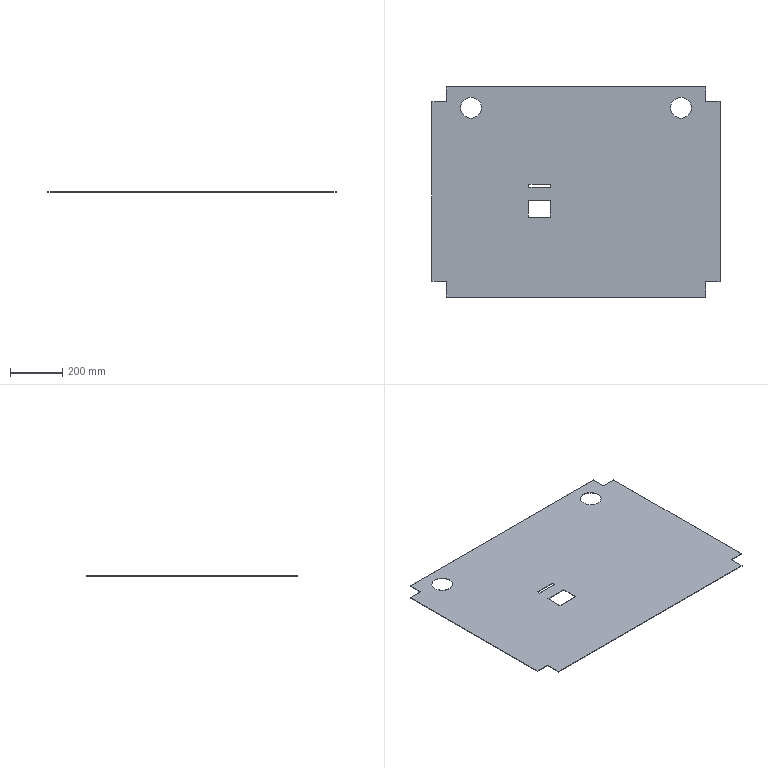Part | SolidWorks | features Cut 2, Extrusion 1 | 1 solid | 26 faces | box 1105 x 806 x 2 mm | volume 1722946 mm3 | plane 22 | cylinder 4 | commonest cylinder face diameters 80 x4
STEP:
#1=CARTESIAN_POINT('',(547.229,80.234,2.));
#2=VERTEX_POINT('',#1);
#3=CARTESIAN_POINT('',(627.229,80.234,2.));
#4=VERTEX_POINT('',#3);
#5=CARTESIAN_POINT('',(587.229,80.234,2.));
#6=DIRECTION('',(0.,0.,1.));
#7=DIRECTION('',(1.,0.,0.));
#8=AXIS2_PLACEMENT_3D('',#5,#6,#7);
#9=CIRCLE('',#8,40.);
#10=EDGE_CURVE('',#2,#4,#9,.T.);
#11=ORIENTED_EDGE('',*,*,#10,.T.);
#12=CARTESIAN_POINT('',(627.229,80.234,0.));
#13=VERTEX_POINT('',#12);
#14=CARTESIAN_POINT('',(627.229,80.234,2.));
#15=DIRECTION('',(0.,0.,-1.));
#16=VECTOR('',#15,1000.);
#17=LINE('',#14,#16);
#18=EDGE_CURVE('',#4,#13,#17,.T.);
#19=ORIENTED_EDGE('',*,*,#18,.T.);
#20=CARTESIAN_POINT('',(547.229,80.234,0.));
#21=VERTEX_POINT('',#20);
#22=CARTESIAN_POINT('',(587.229,80.234,0.));
#23=DIRECTION('',(0.,0.,1.));
#24=DIRECTION('',(1.,0.,0.));
#25=AXIS2_PLACEMENT_3D('',#22,#23,#24);
#26=CIRCLE('',#25,40.);
#27=EDGE_CURVE('',#21,#13,#26,.T.);
#28=ORIENTED_EDGE('',*,*,#27,.F.);
#29=CARTESIAN_POINT('',(547.229,80.234,2.));
#30=DIRECTION('',(0.,0.,-1.));
#31=VECTOR('',#30,1000.);
#32=LINE('',#29,#31);
#33=EDGE_CURVE('',#2,#21,#32,.T.);
#34=ORIENTED_EDGE('',*,*,#33,.F.);
#35=EDGE_LOOP('',(#11,#19,#28,#34));
#36=FACE_OUTER_BOUND('',#35,.T.);
#37=CARTESIAN_POINT('',(587.229,80.234,2.));
#38=DIRECTION('',(0.,0.,-1.));
#39=DIRECTION('',(-1.,0.,0.));
#40=AXIS2_PLACEMENT_3D('',#37,#38,#39);
#41=CYLINDRICAL_SURFACE('',#40,40.);
#42=ADVANCED_FACE('',(#36),#41,.F.);
#43=CARTESIAN_POINT('',(-257.771,80.234,2.));
#44=VERTEX_POINT('',#43);
#45=CARTESIAN_POINT('',(-177.771,80.234,2.));
#46=VERTEX_POINT('',#45);
#47=CARTESIAN_POINT('',(-217.771,80.234,2.));
#48=DIRECTION('',(0.,0.,1.));
#49=DIRECTION('',(1.,0.,0.));
#50=AXIS2_PLACEMENT_3D('',#47,#48,#49);
#51=CIRCLE('',#50,40.);
#52=EDGE_CURVE('',#44,#46,#51,.T.);
#53=ORIENTED_EDGE('',*,*,#52,.T.);
#54=CARTESIAN_POINT('',(-177.771,80.234,0.));
#55=VERTEX_POINT('',#54);
#56=CARTESIAN_POINT('',(-177.771,80.234,2.));
#57=DIRECTION('',(0.,0.,-1.));
#58=VECTOR('',#57,1000.);
#59=LINE('',#56,#58);
#60=EDGE_CURVE('',#46,#55,#59,.T.);
#61=ORIENTED_EDGE('',*,*,#60,.T.);
#62=CARTESIAN_POINT('',(-257.771,80.234,0.));
#63=VERTEX_POINT('',#62);
#64=CARTESIAN_POINT('',(-217.771,80.234,0.));
#65=DIRECTION('',(0.,0.,1.));
#66=DIRECTION('',(1.,0.,0.));
#67=AXIS2_PLACEMENT_3D('',#64,#65,#66);
#68=CIRCLE('',#67,40.);
#69=EDGE_CURVE('',#63,#55,#68,.T.);
#70=ORIENTED_EDGE('',*,*,#69,.F.);
#71=CARTESIAN_POINT('',(-257.771,80.234,2.));
#72=DIRECTION('',(0.,0.,-1.));
#73=VECTOR('',#72,1000.);
#74=LINE('',#71,#73);
#75=EDGE_CURVE('',#44,#63,#74,.T.);
#76=ORIENTED_EDGE('',*,*,#75,.F.);
#77=EDGE_LOOP('',(#53,#61,#70,#76));
#78=FACE_OUTER_BOUND('',#77,.T.);
#79=CARTESIAN_POINT('',(-217.771,80.234,2.));
#80=DIRECTION('',(0.,0.,-1.));
#81=DIRECTION('',(-1.,0.,0.));
#82=AXIS2_PLACEMENT_3D('',#79,#80,#81);
#83=CYLINDRICAL_SURFACE('',#82,40.);
#84=ADVANCED_FACE('',(#78),#83,.F.);
#85=CARTESIAN_POINT('',(1.292,-274.291,2.));
#86=VERTEX_POINT('',#85);
#87=CARTESIAN_POINT('',(86.292,-274.291,2.));
#88=VERTEX_POINT('',#87);
#89=CARTESIAN_POINT('',(46.292,-274.291,2.));
#90=DIRECTION('',(1.,0.,0.));
#91=VECTOR('',#90,1000.);
#92=LINE('',#89,#91);
#93=EDGE_CURVE('',#86,#88,#92,.T.);
#94=ORIENTED_EDGE('',*,*,#93,.T.);
#95=CARTESIAN_POINT('',(86.292,-339.291,2.));
#96=VERTEX_POINT('',#95);
#97=CARTESIAN_POINT('',(86.292,-274.291,2.));
#98=DIRECTION('',(0.,-1.,0.));
#99=VECTOR('',#98,1000.);
#100=LINE('',#97,#99);
#101=EDGE_CURVE('',#88,#96,#100,.T.);
#102=ORIENTED_EDGE('',*,*,#101,.T.);
#103=CARTESIAN_POINT('',(1.292,-339.291,2.));
#104=VERTEX_POINT('',#103);
#105=CARTESIAN_POINT('',(1.292,-339.291,2.));
#106=DIRECTION('',(-1.,0.,0.));
#107=VECTOR('',#106,1000.);
#108=LINE('',#105,#107);
#109=EDGE_CURVE('',#96,#104,#108,.T.);
#110=ORIENTED_EDGE('',*,*,#109,.T.);
#111=CARTESIAN_POINT('',(1.292,-274.291,2.));
#112=DIRECTION('',(0.,1.,0.));
#113=VECTOR('',#112,1000.);
#114=LINE('',#111,#113);
#115=EDGE_CURVE('',#104,#86,#114,.T.);
#116=ORIENTED_EDGE('',*,*,#115,.T.);
#117=EDGE_LOOP('',(#94,#102,#110,#116));
#118=FACE_BOUND('',#117,.T.);
#119=CARTESIAN_POINT('',(4.292,-225.291,2.));
#120=VERTEX_POINT('',#119);
#121=CARTESIAN_POINT('',(4.292,-213.291,2.));
#122=VERTEX_POINT('',#121);
#123=CARTESIAN_POINT('',(4.292,-225.291,2.));
#124=DIRECTION('',(0.,1.,0.));
#125=VECTOR('',#124,1000.);
#126=LINE('',#123,#125);
#127=EDGE_CURVE('',#120,#122,#126,.T.);
#128=ORIENTED_EDGE('',*,*,#127,.T.);
#129=CARTESIAN_POINT('',(86.292,-213.291,2.));
#130=VERTEX_POINT('',#129);
#131=CARTESIAN_POINT('',(4.292,-213.291,2.));
#132=DIRECTION('',(1.,0.,0.));
#133=VECTOR('',#132,1000.);
#134=LINE('',#131,#133);
#135=EDGE_CURVE('',#122,#130,#134,.T.);
#136=ORIENTED_EDGE('',*,*,#135,.T.);
#137=CARTESIAN_POINT('',(86.292,-225.291,2.));
#138=VERTEX_POINT('',#137);
#139=CARTESIAN_POINT('',(86.292,-213.291,2.));
#140=DIRECTION('',(0.,-1.,0.));
#141=VECTOR('',#140,1000.);
#142=LINE('',#139,#141);
#143=EDGE_CURVE('',#130,#138,#142,.T.);
#144=ORIENTED_EDGE('',*,*,#143,.T.);
#145=CARTESIAN_POINT('',(86.292,-225.291,2.));
#146=DIRECTION('',(-1.,0.,0.));
#147=VECTOR('',#146,1000.);
#148=LINE('',#145,#147);
#149=EDGE_CURVE('',#138,#120,#148,.T.);
#150=ORIENTED_EDGE('',*,*,#149,.T.);
#151=EDGE_LOOP('',(#128,#136,#144,#150));
#152=FACE_BOUND('',#151,.T.);
#153=ORIENTED_EDGE('',*,*,#52,.F.);
#154=CARTESIAN_POINT('',(-217.771,80.234,2.));
#155=DIRECTION('',(0.,0.,1.));
#156=DIRECTION('',(1.,0.,0.));
#157=AXIS2_PLACEMENT_3D('',#154,#155,#156);
#158=CIRCLE('',#157,40.);
#159=EDGE_CURVE('',#46,#44,#158,.T.);
#160=ORIENTED_EDGE('',*,*,#159,.F.);
#161=EDGE_LOOP('',(#153,#160));
#162=FACE_BOUND('',#161,.T.);
#163=CARTESIAN_POINT('',(-367.771,104.234,2.));
#164=VERTEX_POINT('',#163);
#165=CARTESIAN_POINT('',(-367.771,-585.766,2.));
#166=VERTEX_POINT('',#165);
#167=CARTESIAN_POINT('',(-367.771,104.234,2.));
#168=DIRECTION('',(0.,-1.,0.));
#169=VECTOR('',#168,1000.);
#170=LINE('',#167,#169);
#171=EDGE_CURVE('',#164,#166,#170,.T.);
#172=ORIENTED_EDGE('',*,*,#171,.T.);
#173=CARTESIAN_POINT('',(-312.771,-585.766,2.));
#174=VERTEX_POINT('',#173);
#175=CARTESIAN_POINT('',(-367.771,-585.766,2.));
#176=DIRECTION('',(1.,0.,0.));
#177=VECTOR('',#176,1000.);
#178=LINE('',#175,#177);
#179=EDGE_CURVE('',#166,#174,#178,.T.);
#180=ORIENTED_EDGE('',*,*,#179,.T.);
#181=CARTESIAN_POINT('',(-312.771,-645.766,2.));
#182=VERTEX_POINT('',#181);
#183=CARTESIAN_POINT('',(-312.771,-585.766,2.));
#184=DIRECTION('',(0.,-1.,0.));
#185=VECTOR('',#184,1000.);
#186=LINE('',#183,#185);
#187=EDGE_CURVE('',#174,#182,#186,.T.);
#188=ORIENTED_EDGE('',*,*,#187,.T.);
#189=CARTESIAN_POINT('',(682.229,-645.766,2.));
#190=VERTEX_POINT('',#189);
#191=CARTESIAN_POINT('',(-312.771,-645.766,2.));
#192=DIRECTION('',(1.,0.,0.));
#193=VECTOR('',#192,1000.);
#194=LINE('',#191,#193);
#195=EDGE_CURVE('',#182,#190,#194,.T.);
#196=ORIENTED_EDGE('',*,*,#195,.T.);
#197=CARTESIAN_POINT('',(682.229,-587.766,2.));
#198=VERTEX_POINT('',#197);
#199=CARTESIAN_POINT('',(682.229,-587.766,2.));
#200=DIRECTION('',(0.,1.,0.));
#201=VECTOR('',#200,1000.);
#202=LINE('',#199,#201);
#203=EDGE_CURVE('',#190,#198,#202,.T.);
#204=ORIENTED_EDGE('',*,*,#203,.T.);
#205=CARTESIAN_POINT('',(737.229,-587.766,2.));
#206=VERTEX_POINT('',#205);
#207=CARTESIAN_POINT('',(737.229,-587.766,2.));
#208=DIRECTION('',(1.,0.,0.));
#209=VECTOR('',#208,1000.);
#210=LINE('',#207,#209);
#211=EDGE_CURVE('',#198,#206,#210,.T.);
#212=ORIENTED_EDGE('',*,*,#211,.T.);
#213=CARTESIAN_POINT('',(737.229,105.234,2.));
#214=VERTEX_POINT('',#213);
#215=CARTESIAN_POINT('',(737.229,105.234,2.));
#216=DIRECTION('',(0.,1.,0.));
#217=VECTOR('',#216,1000.);
#218=LINE('',#215,#217);
#219=EDGE_CURVE('',#206,#214,#218,.T.);
#220=ORIENTED_EDGE('',*,*,#219,.T.);
#221=CARTESIAN_POINT('',(682.229,105.234,2.));
#222=VERTEX_POINT('',#221);
#223=CARTESIAN_POINT('',(737.229,105.234,2.));
#224=DIRECTION('',(-1.,0.,0.));
#225=VECTOR('',#224,1000.);
#226=LINE('',#223,#225);
#227=EDGE_CURVE('',#214,#222,#226,.T.);
#228=ORIENTED_EDGE('',*,*,#227,.T.);
#229=CARTESIAN_POINT('',(682.229,160.234,2.));
#230=VERTEX_POINT('',#229);
#231=CARTESIAN_POINT('',(682.229,105.234,2.));
#232=DIRECTION('',(0.,1.,0.));
#233=VECTOR('',#232,1000.);
#234=LINE('',#231,#233);
#235=EDGE_CURVE('',#222,#230,#234,.T.);
#236=ORIENTED_EDGE('',*,*,#235,.T.);
#237=CARTESIAN_POINT('',(-312.771,160.234,2.));
#238=VERTEX_POINT('',#237);
#239=CARTESIAN_POINT('',(-312.771,160.234,2.));
#240=DIRECTION('',(-1.,0.,0.));
#241=VECTOR('',#240,1000.);
#242=LINE('',#239,#241);
#243=EDGE_CURVE('',#230,#238,#242,.T.);
#244=ORIENTED_EDGE('',*,*,#243,.T.);
#245=CARTESIAN_POINT('',(-312.771,104.234,2.));
#246=VERTEX_POINT('',#245);
#247=CARTESIAN_POINT('',(-312.771,104.234,2.));
#248=DIRECTION('',(0.,-1.,0.));
#249=VECTOR('',#248,1000.);
#250=LINE('',#247,#249);
#251=EDGE_CURVE('',#238,#246,#250,.T.);
#252=ORIENTED_EDGE('',*,*,#251,.T.);
#253=CARTESIAN_POINT('',(-367.771,104.234,2.));
#254=DIRECTION('',(-1.,0.,0.));
#255=VECTOR('',#254,1000.);
#256=LINE('',#253,#255);
#257=EDGE_CURVE('',#246,#164,#256,.T.);
#258=ORIENTED_EDGE('',*,*,#257,.T.);
#259=EDGE_LOOP('',(#172,#180,#188,#196,#204,#212,#220,#228,#236,#244,#252,#258));
#260=FACE_OUTER_BOUND('',#259,.T.);
#261=ORIENTED_EDGE('',*,*,#10,.F.);
#262=CARTESIAN_POINT('',(587.229,80.234,2.));
#263=DIRECTION('',(0.,0.,1.));
#264=DIRECTION('',(1.,0.,0.));
#265=AXIS2_PLACEMENT_3D('',#262,#263,#264);
#266=CIRCLE('',#265,40.);
#267=EDGE_CURVE('',#4,#2,#266,.T.);
#268=ORIENTED_EDGE('',*,*,#267,.F.);
#269=EDGE_LOOP('',(#261,#268));
#270=FACE_BOUND('',#269,.T.);
#271=CARTESIAN_POINT('',(0.,0.,2.));
#272=DIRECTION('',(0.,0.,1.));
#273=DIRECTION('',(1.,0.,0.));
#274=AXIS2_PLACEMENT_3D('',#271,#272,#273);
#275=PLANE('',#274);
#276=ADVANCED_FACE('',(#118,#152,#162,#260,#270),#275,.T.);
#277=CARTESIAN_POINT('',(86.292,-274.291,0.));
#278=VERTEX_POINT('',#277);
#279=CARTESIAN_POINT('',(86.292,-339.291,0.));
#280=VERTEX_POINT('',#279);
#281=CARTESIAN_POINT('',(86.292,-274.291,0.));
#282=DIRECTION('',(0.,-1.,0.));
#283=VECTOR('',#282,1000.);
#284=LINE('',#281,#283);
#285=EDGE_CURVE('',#278,#280,#284,.T.);
#286=ORIENTED_EDGE('',*,*,#285,.F.);
#287=CARTESIAN_POINT('',(1.292,-274.291,0.));
#288=VERTEX_POINT('',#287);
#289=CARTESIAN_POINT('',(46.292,-274.291,0.));
#290=DIRECTION('',(1.,0.,0.));
#291=VECTOR('',#290,1000.);
#292=LINE('',#289,#291);
#293=EDGE_CURVE('',#288,#278,#292,.T.);
#294=ORIENTED_EDGE('',*,*,#293,.F.);
#295=CARTESIAN_POINT('',(1.292,-339.291,0.));
#296=VERTEX_POINT('',#295);
#297=CARTESIAN_POINT('',(1.292,-274.291,0.));
#298=DIRECTION('',(0.,1.,0.));
#299=VECTOR('',#298,1000.);
#300=LINE('',#297,#299);
#301=EDGE_CURVE('',#296,#288,#300,.T.);
#302=ORIENTED_EDGE('',*,*,#301,.F.);
#303=CARTESIAN_POINT('',(1.292,-339.291,0.));
#304=DIRECTION('',(-1.,0.,0.));
#305=VECTOR('',#304,1000.);
#306=LINE('',#303,#305);
#307=EDGE_CURVE('',#280,#296,#306,.T.);
#308=ORIENTED_EDGE('',*,*,#307,.F.);
#309=EDGE_LOOP('',(#286,#294,#302,#308));
#310=FACE_BOUND('',#309,.T.);
#311=CARTESIAN_POINT('',(4.292,-213.291,0.));
#312=VERTEX_POINT('',#311);
#313=CARTESIAN_POINT('',(86.292,-213.291,0.));
#314=VERTEX_POINT('',#313);
#315=CARTESIAN_POINT('',(4.292,-213.291,0.));
#316=DIRECTION('',(1.,0.,0.));
#317=VECTOR('',#316,1000.);
#318=LINE('',#315,#317);
#319=EDGE_CURVE('',#312,#314,#318,.T.);
#320=ORIENTED_EDGE('',*,*,#319,.F.);
#321=CARTESIAN_POINT('',(4.292,-225.291,0.));
#322=VERTEX_POINT('',#321);
#323=CARTESIAN_POINT('',(4.292,-225.291,0.));
#324=DIRECTION('',(0.,1.,0.));
#325=VECTOR('',#324,1000.);
#326=LINE('',#323,#325);
#327=EDGE_CURVE('',#322,#312,#326,.T.);
#328=ORIENTED_EDGE('',*,*,#327,.F.);
#329=CARTESIAN_POINT('',(86.292,-225.291,0.));
#330=VERTEX_POINT('',#329);
#331=CARTESIAN_POINT('',(86.292,-225.291,0.));
#332=DIRECTION('',(-1.,0.,0.));
#333=VECTOR('',#332,1000.);
#334=LINE('',#331,#333);
#335=EDGE_CURVE('',#330,#322,#334,.T.);
#336=ORIENTED_EDGE('',*,*,#335,.F.);
#337=CARTESIAN_POINT('',(86.292,-213.291,0.));
#338=DIRECTION('',(0.,-1.,0.));
#339=VECTOR('',#338,1000.);
#340=LINE('',#337,#339);
#341=EDGE_CURVE('',#314,#330,#340,.T.);
#342=ORIENTED_EDGE('',*,*,#341,.F.);
#343=EDGE_LOOP('',(#320,#328,#336,#342));
#344=FACE_BOUND('',#343,.T.);
#345=CARTESIAN_POINT('',(-367.771,104.234,0.));
#346=VERTEX_POINT('',#345);
#347=CARTESIAN_POINT('',(-367.771,-585.766,0.));
#348=VERTEX_POINT('',#347);
#349=CARTESIAN_POINT('',(-367.771,104.234,0.));
#350=DIRECTION('',(0.,-1.,0.));
#351=VECTOR('',#350,1000.);
#352=LINE('',#349,#351);
#353=EDGE_CURVE('',#346,#348,#352,.T.);
#354=ORIENTED_EDGE('',*,*,#353,.F.);
#355=CARTESIAN_POINT('',(-312.771,104.234,0.));
#356=VERTEX_POINT('',#355);
#357=CARTESIAN_POINT('',(-367.771,104.234,0.));
#358=DIRECTION('',(-1.,0.,0.));
#359=VECTOR('',#358,1000.);
#360=LINE('',#357,#359);
#361=EDGE_CURVE('',#356,#346,#360,.T.);
#362=ORIENTED_EDGE('',*,*,#361,.F.);
#363=CARTESIAN_POINT('',(-312.771,160.234,0.));
#364=VERTEX_POINT('',#363);
#365=CARTESIAN_POINT('',(-312.771,104.234,0.));
#366=DIRECTION('',(0.,-1.,0.));
#367=VECTOR('',#366,1000.);
#368=LINE('',#365,#367);
#369=EDGE_CURVE('',#364,#356,#368,.T.);
#370=ORIENTED_EDGE('',*,*,#369,.F.);
#371=CARTESIAN_POINT('',(682.229,160.234,0.));
#372=VERTEX_POINT('',#371);
#373=CARTESIAN_POINT('',(-312.771,160.234,0.));
#374=DIRECTION('',(-1.,0.,0.));
#375=VECTOR('',#374,1000.);
#376=LINE('',#373,#375);
#377=EDGE_CURVE('',#372,#364,#376,.T.);
#378=ORIENTED_EDGE('',*,*,#377,.F.);
#379=CARTESIAN_POINT('',(682.229,105.234,0.));
#380=VERTEX_POINT('',#379);
#381=CARTESIAN_POINT('',(682.229,105.234,0.));
#382=DIRECTION('',(0.,1.,0.));
#383=VECTOR('',#382,1000.);
#384=LINE('',#381,#383);
#385=EDGE_CURVE('',#380,#372,#384,.T.);
#386=ORIENTED_EDGE('',*,*,#385,.F.);
#387=CARTESIAN_POINT('',(737.229,105.234,0.));
#388=VERTEX_POINT('',#387);
#389=CARTESIAN_POINT('',(737.229,105.234,0.));
#390=DIRECTION('',(-1.,0.,0.));
#391=VECTOR('',#390,1000.);
#392=LINE('',#389,#391);
#393=EDGE_CURVE('',#388,#380,#392,.T.);
#394=ORIENTED_EDGE('',*,*,#393,.F.);
#395=CARTESIAN_POINT('',(737.229,-587.766,0.));
#396=VERTEX_POINT('',#395);
#397=CARTESIAN_POINT('',(737.229,105.234,0.));
#398=DIRECTION('',(0.,1.,0.));
#399=VECTOR('',#398,1000.);
#400=LINE('',#397,#399);
#401=EDGE_CURVE('',#396,#388,#400,.T.);
#402=ORIENTED_EDGE('',*,*,#401,.F.);
#403=CARTESIAN_POINT('',(682.229,-587.766,0.));
#404=VERTEX_POINT('',#403);
#405=CARTESIAN_POINT('',(737.229,-587.766,0.));
#406=DIRECTION('',(1.,0.,0.));
#407=VECTOR('',#406,1000.);
#408=LINE('',#405,#407);
#409=EDGE_CURVE('',#404,#396,#408,.T.);
#410=ORIENTED_EDGE('',*,*,#409,.F.);
#411=CARTESIAN_POINT('',(682.229,-645.766,0.));
#412=VERTEX_POINT('',#411);
#413=CARTESIAN_POINT('',(682.229,-587.766,0.));
#414=DIRECTION('',(0.,1.,0.));
#415=VECTOR('',#414,1000.);
#416=LINE('',#413,#415);
#417=EDGE_CURVE('',#412,#404,#416,.T.);
#418=ORIENTED_EDGE('',*,*,#417,.F.);
#419=CARTESIAN_POINT('',(-312.771,-645.766,0.));
#420=VERTEX_POINT('',#419);
#421=CARTESIAN_POINT('',(-312.771,-645.766,0.));
#422=DIRECTION('',(1.,0.,0.));
#423=VECTOR('',#422,1000.);
#424=LINE('',#421,#423);
#425=EDGE_CURVE('',#420,#412,#424,.T.);
#426=ORIENTED_EDGE('',*,*,#425,.F.);
#427=CARTESIAN_POINT('',(-312.771,-585.766,0.));
#428=VERTEX_POINT('',#427);
#429=CARTESIAN_POINT('',(-312.771,-585.766,0.));
#430=DIRECTION('',(0.,-1.,0.));
#431=VECTOR('',#430,1000.);
#432=LINE('',#429,#431);
#433=EDGE_CURVE('',#428,#420,#432,.T.);
#434=ORIENTED_EDGE('',*,*,#433,.F.);
#435=CARTESIAN_POINT('',(-367.771,-585.766,0.));
#436=DIRECTION('',(1.,0.,0.));
#437=VECTOR('',#436,1000.);
#438=LINE('',#435,#437);
#439=EDGE_CURVE('',#348,#428,#438,.T.);
#440=ORIENTED_EDGE('',*,*,#439,.F.);
#441=EDGE_LOOP('',(#354,#362,#370,#378,#386,#394,#402,#410,#418,#426,#434,#440));
#442=FACE_OUTER_BOUND('',#441,.T.);
#443=ORIENTED_EDGE('',*,*,#69,.T.);
#444=CARTESIAN_POINT('',(-217.771,80.234,0.));
#445=DIRECTION('',(0.,0.,1.));
#446=DIRECTION('',(1.,0.,0.));
#447=AXIS2_PLACEMENT_3D('',#444,#445,#446);
#448=CIRCLE('',#447,40.);
#449=EDGE_CURVE('',#55,#63,#448,.T.);
#450=ORIENTED_EDGE('',*,*,#449,.T.);
#451=EDGE_LOOP('',(#443,#450));
#452=FACE_BOUND('',#451,.T.);
#453=ORIENTED_EDGE('',*,*,#27,.T.);
#454=CARTESIAN_POINT('',(587.229,80.234,0.));
#455=DIRECTION('',(0.,0.,1.));
#456=DIRECTION('',(1.,0.,0.));
#457=AXIS2_PLACEMENT_3D('',#454,#455,#456);
#458=CIRCLE('',#457,40.);
#459=EDGE_CURVE('',#13,#21,#458,.T.);
#460=ORIENTED_EDGE('',*,*,#459,.T.);
#461=EDGE_LOOP('',(#453,#460));
#462=FACE_BOUND('',#461,.T.);
#463=CARTESIAN_POINT('',(0.,0.,0.));
#464=DIRECTION('',(0.,0.,1.));
#465=DIRECTION('',(1.,0.,0.));
#466=AXIS2_PLACEMENT_3D('',#463,#464,#465);
#467=PLANE('',#466);
#468=ADVANCED_FACE('',(#310,#344,#442,#452,#462),#467,.F.);
#469=ORIENTED_EDGE('',*,*,#353,.T.);
#470=CARTESIAN_POINT('',(-367.771,-585.766,2.));
#471=DIRECTION('',(0.,0.,-1.));
#472=VECTOR('',#471,1000.);
#473=LINE('',#470,#472);
#474=EDGE_CURVE('',#166,#348,#473,.T.);
#475=ORIENTED_EDGE('',*,*,#474,.F.);
#476=ORIENTED_EDGE('',*,*,#171,.F.);
#477=CARTESIAN_POINT('',(-367.771,104.234,2.));
#478=DIRECTION('',(0.,0.,-1.));
#479=VECTOR('',#478,1000.);
#480=LINE('',#477,#479);
#481=EDGE_CURVE('',#164,#346,#480,.T.);
#482=ORIENTED_EDGE('',*,*,#481,.T.);
#483=EDGE_LOOP('',(#469,#475,#476,#482));
#484=FACE_OUTER_BOUND('',#483,.T.);
#485=CARTESIAN_POINT('',(-367.771,104.234,2.));
#486=DIRECTION('',(1.,0.,0.));
#487=DIRECTION('',(0.,0.,-1.));
#488=AXIS2_PLACEMENT_3D('',#485,#486,#487);
#489=PLANE('',#488);
#490=ADVANCED_FACE('',(#484),#489,.F.);
#491=ORIENTED_EDGE('',*,*,#439,.T.);
#492=CARTESIAN_POINT('',(-312.771,-585.766,2.));
#493=DIRECTION('',(0.,0.,-1.));
#494=VECTOR('',#493,1000.);
#495=LINE('',#492,#494);
#496=EDGE_CURVE('',#174,#428,#495,.T.);
#497=ORIENTED_EDGE('',*,*,#496,.F.);
#498=ORIENTED_EDGE('',*,*,#179,.F.);
#499=ORIENTED_EDGE('',*,*,#474,.T.);
#500=EDGE_LOOP('',(#491,#497,#498,#499));
#501=FACE_OUTER_BOUND('',#500,.T.);
#502=CARTESIAN_POINT('',(-367.771,-585.766,2.));
#503=DIRECTION('',(0.,1.,0.));
#504=DIRECTION('',(0.,0.,1.));
#505=AXIS2_PLACEMENT_3D('',#502,#503,#504);
#506=PLANE('',#505);
#507=ADVANCED_FACE('',(#501),#506,.F.);
#508=ORIENTED_EDGE('',*,*,#433,.T.);
#509=CARTESIAN_POINT('',(-312.771,-645.766,2.));
#510=DIRECTION('',(0.,0.,-1.));
#511=VECTOR('',#510,1000.);
#512=LINE('',#509,#511);
#513=EDGE_CURVE('',#182,#420,#512,.T.);
#514=ORIENTED_EDGE('',*,*,#513,.F.);
#515=ORIENTED_EDGE('',*,*,#187,.F.);
#516=ORIENTED_EDGE('',*,*,#496,.T.);
#517=EDGE_LOOP('',(#508,#514,#515,#516));
#518=FACE_OUTER_BOUND('',#517,.T.);
#519=CARTESIAN_POINT('',(-312.771,-585.766,2.));
#520=DIRECTION('',(1.,0.,0.));
#521=DIRECTION('',(0.,0.,-1.));
#522=AXIS2_PLACEMENT_3D('',#519,#520,#521);
#523=PLANE('',#522);
#524=ADVANCED_FACE('',(#518),#523,.F.);
#525=ORIENTED_EDGE('',*,*,#425,.T.);
#526=CARTESIAN_POINT('',(682.229,-645.766,2.));
#527=DIRECTION('',(0.,0.,-1.));
#528=VECTOR('',#527,1000.);
#529=LINE('',#526,#528);
#530=EDGE_CURVE('',#190,#412,#529,.T.);
#531=ORIENTED_EDGE('',*,*,#530,.F.);
#532=ORIENTED_EDGE('',*,*,#195,.F.);
#533=ORIENTED_EDGE('',*,*,#513,.T.);
#534=EDGE_LOOP('',(#525,#531,#532,#533));
#535=FACE_OUTER_BOUND('',#534,.T.);
#536=CARTESIAN_POINT('',(-312.771,-645.766,2.));
#537=DIRECTION('',(0.,1.,0.));
#538=DIRECTION('',(-1.,0.,0.));
#539=AXIS2_PLACEMENT_3D('',#536,#537,#538);
#540=PLANE('',#539);
#541=ADVANCED_FACE('',(#535),#540,.F.);
#542=ORIENTED_EDGE('',*,*,#417,.T.);
#543=CARTESIAN_POINT('',(682.229,-587.766,2.));
#544=DIRECTION('',(0.,0.,-1.));
#545=VECTOR('',#544,1000.);
#546=LINE('',#543,#545);
#547=EDGE_CURVE('',#198,#404,#546,.T.);
#548=ORIENTED_EDGE('',*,*,#547,.F.);
#549=ORIENTED_EDGE('',*,*,#203,.F.);
#550=ORIENTED_EDGE('',*,*,#530,.T.);
#551=EDGE_LOOP('',(#542,#548,#549,#550));
#552=FACE_OUTER_BOUND('',#551,.T.);
#553=CARTESIAN_POINT('',(682.229,-587.766,2.));
#554=DIRECTION('',(-1.,0.,0.));
#555=DIRECTION('',(0.,0.,1.));
#556=AXIS2_PLACEMENT_3D('',#553,#554,#555);
#557=PLANE('',#556);
#558=ADVANCED_FACE('',(#552),#557,.F.);
#559=ORIENTED_EDGE('',*,*,#409,.T.);
#560=CARTESIAN_POINT('',(737.229,-587.766,2.));
#561=DIRECTION('',(0.,0.,-1.));
#562=VECTOR('',#561,1000.);
#563=LINE('',#560,#562);
#564=EDGE_CURVE('',#206,#396,#563,.T.);
#565=ORIENTED_EDGE('',*,*,#564,.F.);
#566=ORIENTED_EDGE('',*,*,#211,.F.);
#567=ORIENTED_EDGE('',*,*,#547,.T.);
#568=EDGE_LOOP('',(#559,#565,#566,#567));
#569=FACE_OUTER_BOUND('',#568,.T.);
#570=CARTESIAN_POINT('',(737.229,-587.766,2.));
#571=DIRECTION('',(0.,1.,0.));
#572=DIRECTION('',(0.,0.,1.));
#573=AXIS2_PLACEMENT_3D('',#570,#571,#572);
#574=PLANE('',#573);
#575=ADVANCED_FACE('',(#569),#574,.F.);
#576=ORIENTED_EDGE('',*,*,#401,.T.);
#577=CARTESIAN_POINT('',(737.229,105.234,2.));
#578=DIRECTION('',(0.,0.,-1.));
#579=VECTOR('',#578,1000.);
#580=LINE('',#577,#579);
#581=EDGE_CURVE('',#214,#388,#580,.T.);
#582=ORIENTED_EDGE('',*,*,#581,.F.);
#583=ORIENTED_EDGE('',*,*,#219,.F.);
#584=ORIENTED_EDGE('',*,*,#564,.T.);
#585=EDGE_LOOP('',(#576,#582,#583,#584));
#586=FACE_OUTER_BOUND('',#585,.T.);
#587=CARTESIAN_POINT('',(737.229,105.234,2.));
#588=DIRECTION('',(-1.,0.,0.));
#589=DIRECTION('',(0.,-1.,0.));
#590=AXIS2_PLACEMENT_3D('',#587,#588,#589);
#591=PLANE('',#590);
#592=ADVANCED_FACE('',(#586),#591,.F.);
#593=ORIENTED_EDGE('',*,*,#393,.T.);
#594=CARTESIAN_POINT('',(682.229,105.234,2.));
#595=DIRECTION('',(0.,0.,-1.));
#596=VECTOR('',#595,1000.);
#597=LINE('',#594,#596);
#598=EDGE_CURVE('',#222,#380,#597,.T.);
#599=ORIENTED_EDGE('',*,*,#598,.F.);
#600=ORIENTED_EDGE('',*,*,#227,.F.);
#601=ORIENTED_EDGE('',*,*,#581,.T.);
#602=EDGE_LOOP('',(#593,#599,#600,#601));
#603=FACE_OUTER_BOUND('',#602,.T.);
#604=CARTESIAN_POINT('',(737.229,105.234,2.));
#605=DIRECTION('',(0.,-1.,0.));
#606=DIRECTION('',(1.,0.,0.));
#607=AXIS2_PLACEMENT_3D('',#604,#605,#606);
#608=PLANE('',#607);
#609=ADVANCED_FACE('',(#603),#608,.F.);
#610=ORIENTED_EDGE('',*,*,#385,.T.);
#611=CARTESIAN_POINT('',(682.229,160.234,2.));
#612=DIRECTION('',(0.,0.,-1.));
#613=VECTOR('',#612,1000.);
#614=LINE('',#611,#613);
#615=EDGE_CURVE('',#230,#372,#614,.T.);
#616=ORIENTED_EDGE('',*,*,#615,.F.);
#617=ORIENTED_EDGE('',*,*,#235,.F.);
#618=ORIENTED_EDGE('',*,*,#598,.T.);
#619=EDGE_LOOP('',(#610,#616,#617,#618));
#620=FACE_OUTER_BOUND('',#619,.T.);
#621=CARTESIAN_POINT('',(682.229,105.234,2.));
#622=DIRECTION('',(-1.,0.,0.));
#623=DIRECTION('',(0.,-1.,0.));
#624=AXIS2_PLACEMENT_3D('',#621,#622,#623);
#625=PLANE('',#624);
#626=ADVANCED_FACE('',(#620),#625,.F.);
#627=ORIENTED_EDGE('',*,*,#377,.T.);
#628=CARTESIAN_POINT('',(-312.771,160.234,2.));
#629=DIRECTION('',(0.,0.,-1.));
#630=VECTOR('',#629,1000.);
#631=LINE('',#628,#630);
#632=EDGE_CURVE('',#238,#364,#631,.T.);
#633=ORIENTED_EDGE('',*,*,#632,.F.);
#634=ORIENTED_EDGE('',*,*,#243,.F.);
#635=ORIENTED_EDGE('',*,*,#615,.T.);
#636=EDGE_LOOP('',(#627,#633,#634,#635));
#637=FACE_OUTER_BOUND('',#636,.T.);
#638=CARTESIAN_POINT('',(-312.771,160.234,2.));
#639=DIRECTION('',(0.,-1.,0.));
#640=DIRECTION('',(1.,0.,0.));
#641=AXIS2_PLACEMENT_3D('',#638,#639,#640);
#642=PLANE('',#641);
#643=ADVANCED_FACE('',(#637),#642,.F.);
#644=ORIENTED_EDGE('',*,*,#369,.T.);
#645=CARTESIAN_POINT('',(-312.771,104.234,2.));
#646=DIRECTION('',(0.,0.,-1.));
#647=VECTOR('',#646,1000.);
#648=LINE('',#645,#647);
#649=EDGE_CURVE('',#246,#356,#648,.T.);
#650=ORIENTED_EDGE('',*,*,#649,.F.);
#651=ORIENTED_EDGE('',*,*,#251,.F.);
#652=ORIENTED_EDGE('',*,*,#632,.T.);
#653=EDGE_LOOP('',(#644,#650,#651,#652));
#654=FACE_OUTER_BOUND('',#653,.T.);
#655=CARTESIAN_POINT('',(-312.771,104.234,2.));
#656=DIRECTION('',(1.,0.,0.));
#657=DIRECTION('',(0.,0.,-1.));
#658=AXIS2_PLACEMENT_3D('',#655,#656,#657);
#659=PLANE('',#658);
#660=ADVANCED_FACE('',(#654),#659,.F.);
#661=ORIENTED_EDGE('',*,*,#361,.T.);
#662=ORIENTED_EDGE('',*,*,#481,.F.);
#663=ORIENTED_EDGE('',*,*,#257,.F.);
#664=ORIENTED_EDGE('',*,*,#649,.T.);
#665=EDGE_LOOP('',(#661,#662,#663,#664));
#666=FACE_OUTER_BOUND('',#665,.T.);
#667=CARTESIAN_POINT('',(-367.771,104.234,2.));
#668=DIRECTION('',(0.,-1.,0.));
#669=DIRECTION('',(0.,0.,-1.));
#670=AXIS2_PLACEMENT_3D('',#667,#668,#669);
#671=PLANE('',#670);
#672=ADVANCED_FACE('',(#666),#671,.F.);
#673=ORIENTED_EDGE('',*,*,#60,.F.);
#674=ORIENTED_EDGE('',*,*,#159,.T.);
#675=ORIENTED_EDGE('',*,*,#75,.T.);
#676=ORIENTED_EDGE('',*,*,#449,.F.);
#677=EDGE_LOOP('',(#673,#674,#675,#676));
#678=FACE_OUTER_BOUND('',#677,.T.);
#679=CARTESIAN_POINT('',(-217.771,80.234,2.));
#680=DIRECTION('',(0.,0.,-1.));
#681=DIRECTION('',(-1.,0.,0.));
#682=AXIS2_PLACEMENT_3D('',#679,#680,#681);
#683=CYLINDRICAL_SURFACE('',#682,40.);
#684=ADVANCED_FACE('',(#678),#683,.F.);
#685=ORIENTED_EDGE('',*,*,#18,.F.);
#686=ORIENTED_EDGE('',*,*,#267,.T.);
#687=ORIENTED_EDGE('',*,*,#33,.T.);
#688=ORIENTED_EDGE('',*,*,#459,.F.);
#689=EDGE_LOOP('',(#685,#686,#687,#688));
#690=FACE_OUTER_BOUND('',#689,.T.);
#691=CARTESIAN_POINT('',(587.229,80.234,2.));
#692=DIRECTION('',(0.,0.,-1.));
#693=DIRECTION('',(-1.,0.,0.));
#694=AXIS2_PLACEMENT_3D('',#691,#692,#693);
#695=CYLINDRICAL_SURFACE('',#694,40.);
#696=ADVANCED_FACE('',(#690),#695,.F.);
#697=ORIENTED_EDGE('',*,*,#327,.T.);
#698=CARTESIAN_POINT('',(4.292,-213.291,2.));
#699=DIRECTION('',(0.,0.,-1.));
#700=VECTOR('',#699,1000.);
#701=LINE('',#698,#700);
#702=EDGE_CURVE('',#122,#312,#701,.T.);
#703=ORIENTED_EDGE('',*,*,#702,.F.);
#704=ORIENTED_EDGE('',*,*,#127,.F.);
#705=CARTESIAN_POINT('',(4.292,-225.291,2.));
#706=DIRECTION('',(0.,0.,-1.));
#707=VECTOR('',#706,1000.);
#708=LINE('',#705,#707);
#709=EDGE_CURVE('',#120,#322,#708,.T.);
#710=ORIENTED_EDGE('',*,*,#709,.T.);
#711=EDGE_LOOP('',(#697,#703,#704,#710));
#712=FACE_OUTER_BOUND('',#711,.T.);
#713=CARTESIAN_POINT('',(4.292,-225.291,2.));
#714=DIRECTION('',(-1.,0.,0.));
#715=DIRECTION('',(0.,0.,1.));
#716=AXIS2_PLACEMENT_3D('',#713,#714,#715);
#717=PLANE('',#716);
#718=ADVANCED_FACE('',(#712),#717,.F.);
#719=ORIENTED_EDGE('',*,*,#335,.T.);
#720=ORIENTED_EDGE('',*,*,#709,.F.);
#721=ORIENTED_EDGE('',*,*,#149,.F.);
#722=CARTESIAN_POINT('',(86.292,-225.291,2.));
#723=DIRECTION('',(0.,0.,-1.));
#724=VECTOR('',#723,1000.);
#725=LINE('',#722,#724);
#726=EDGE_CURVE('',#138,#330,#725,.T.);
#727=ORIENTED_EDGE('',*,*,#726,.T.);
#728=EDGE_LOOP('',(#719,#720,#721,#727));
#729=FACE_OUTER_BOUND('',#728,.T.);
#730=CARTESIAN_POINT('',(86.292,-225.291,2.));
#731=DIRECTION('',(0.,-1.,0.));
#732=DIRECTION('',(0.,0.,-1.));
#733=AXIS2_PLACEMENT_3D('',#730,#731,#732);
#734=PLANE('',#733);
#735=ADVANCED_FACE('',(#729),#734,.F.);
#736=ORIENTED_EDGE('',*,*,#341,.T.);
#737=ORIENTED_EDGE('',*,*,#726,.F.);
#738=ORIENTED_EDGE('',*,*,#143,.F.);
#739=CARTESIAN_POINT('',(86.292,-213.291,2.));
#740=DIRECTION('',(0.,0.,-1.));
#741=VECTOR('',#740,1000.);
#742=LINE('',#739,#741);
#743=EDGE_CURVE('',#130,#314,#742,.T.);
#744=ORIENTED_EDGE('',*,*,#743,.T.);
#745=EDGE_LOOP('',(#736,#737,#738,#744));
#746=FACE_OUTER_BOUND('',#745,.T.);
#747=CARTESIAN_POINT('',(86.292,-213.291,2.));
#748=DIRECTION('',(1.,0.,0.));
#749=DIRECTION('',(0.,0.,-1.));
#750=AXIS2_PLACEMENT_3D('',#747,#748,#749);
#751=PLANE('',#750);
#752=ADVANCED_FACE('',(#746),#751,.F.);
#753=ORIENTED_EDGE('',*,*,#319,.T.);
#754=ORIENTED_EDGE('',*,*,#743,.F.);
#755=ORIENTED_EDGE('',*,*,#135,.F.);
#756=ORIENTED_EDGE('',*,*,#702,.T.);
#757=EDGE_LOOP('',(#753,#754,#755,#756));
#758=FACE_OUTER_BOUND('',#757,.T.);
#759=CARTESIAN_POINT('',(4.292,-213.291,2.));
#760=DIRECTION('',(0.,1.,0.));
#761=DIRECTION('',(0.,0.,1.));
#762=AXIS2_PLACEMENT_3D('',#759,#760,#761);
#763=PLANE('',#762);
#764=ADVANCED_FACE('',(#758),#763,.F.);
#765=CARTESIAN_POINT('',(1.292,-274.291,109.005));
#766=DIRECTION('',(0.,0.,-1.));
#767=VECTOR('',#766,1000.);
#768=LINE('',#765,#767);
#769=EDGE_CURVE('',#86,#288,#768,.T.);
#770=ORIENTED_EDGE('',*,*,#769,.T.);
#771=ORIENTED_EDGE('',*,*,#293,.T.);
#772=CARTESIAN_POINT('',(86.292,-274.291,109.005));
#773=DIRECTION('',(0.,0.,-1.));
#774=VECTOR('',#773,1000.);
#775=LINE('',#772,#774);
#776=EDGE_CURVE('',#88,#278,#775,.T.);
#777=ORIENTED_EDGE('',*,*,#776,.F.);
#778=ORIENTED_EDGE('',*,*,#93,.F.);
#779=EDGE_LOOP('',(#770,#771,#777,#778));
#780=FACE_OUTER_BOUND('',#779,.T.);
#781=CARTESIAN_POINT('',(46.292,-274.291,109.005));
#782=DIRECTION('',(0.,1.,0.));
#783=DIRECTION('',(0.,0.,1.));
#784=AXIS2_PLACEMENT_3D('',#781,#782,#783);
#785=PLANE('',#784);
#786=ADVANCED_FACE('',(#780),#785,.F.);
#787=ORIENTED_EDGE('',*,*,#776,.T.);
#788=ORIENTED_EDGE('',*,*,#285,.T.);
#789=CARTESIAN_POINT('',(86.292,-339.291,109.005));
#790=DIRECTION('',(0.,0.,-1.));
#791=VECTOR('',#790,1000.);
#792=LINE('',#789,#791);
#793=EDGE_CURVE('',#96,#280,#792,.T.);
#794=ORIENTED_EDGE('',*,*,#793,.F.);
#795=ORIENTED_EDGE('',*,*,#101,.F.);
#796=EDGE_LOOP('',(#787,#788,#794,#795));
#797=FACE_OUTER_BOUND('',#796,.T.);
#798=CARTESIAN_POINT('',(86.292,-274.291,109.005));
#799=DIRECTION('',(1.,0.,0.));
#800=DIRECTION('',(0.,0.,-1.));
#801=AXIS2_PLACEMENT_3D('',#798,#799,#800);
#802=PLANE('',#801);
#803=ADVANCED_FACE('',(#797),#802,.F.);
#804=ORIENTED_EDGE('',*,*,#793,.T.);
#805=ORIENTED_EDGE('',*,*,#307,.T.);
#806=CARTESIAN_POINT('',(1.292,-339.291,109.005));
#807=DIRECTION('',(0.,0.,-1.));
#808=VECTOR('',#807,1000.);
#809=LINE('',#806,#808);
#810=EDGE_CURVE('',#104,#296,#809,.T.);
#811=ORIENTED_EDGE('',*,*,#810,.F.);
#812=ORIENTED_EDGE('',*,*,#109,.F.);
#813=EDGE_LOOP('',(#804,#805,#811,#812));
#814=FACE_OUTER_BOUND('',#813,.T.);
#815=CARTESIAN_POINT('',(1.292,-339.291,109.005));
#816=DIRECTION('',(0.,-1.,0.));
#817=DIRECTION('',(0.,0.,-1.));
#818=AXIS2_PLACEMENT_3D('',#815,#816,#817);
#819=PLANE('',#818);
#820=ADVANCED_FACE('',(#814),#819,.F.);
#821=ORIENTED_EDGE('',*,*,#810,.T.);
#822=ORIENTED_EDGE('',*,*,#301,.T.);
#823=ORIENTED_EDGE('',*,*,#769,.F.);
#824=ORIENTED_EDGE('',*,*,#115,.F.);
#825=EDGE_LOOP('',(#821,#822,#823,#824));
#826=FACE_OUTER_BOUND('',#825,.T.);
#827=CARTESIAN_POINT('',(1.292,-274.291,109.005));
#828=DIRECTION('',(-1.,0.,0.));
#829=DIRECTION('',(0.,0.,1.));
#830=AXIS2_PLACEMENT_3D('',#827,#828,#829);
#831=PLANE('',#830);
#832=ADVANCED_FACE('',(#826),#831,.F.);
#833=CLOSED_SHELL('',(#42,#84,#276,#468,#490,#507,#524,#541,#558,#575,#592,#609,#626,#643,#660,#672,#684,#696,#718,#735,#752,#764,#786,#803,#820,#832));
#834=MANIFOLD_SOLID_BREP('',#833);
#835=CARTESIAN_POINT('',(0.,0.,0.));
#836=DIRECTION('',(0.,0.,1.));
#837=DIRECTION('',(1.,0.,0.));
#838=AXIS2_PLACEMENT_3D('',#835,#836,#837);
#839=(LENGTH_UNIT()NAMED_UNIT(*)SI_UNIT(.MILLI.,.METRE.));
#840=UNCERTAINTY_MEASURE_WITH_UNIT(LENGTH_MEASURE(0.00001),#839,'','');
#841=(NAMED_UNIT(*)PLANE_ANGLE_UNIT()SI_UNIT($,.RADIAN.));
#842=(NAMED_UNIT(*)SI_UNIT($,.STERADIAN.)SOLID_ANGLE_UNIT());
#843=(GEOMETRIC_REPRESENTATION_CONTEXT(3)GLOBAL_UNCERTAINTY_ASSIGNED_CONTEXT((#840))GLOBAL_UNIT_ASSIGNED_CONTEXT((#839,#841,#842))REPRESENTATION_CONTEXT('',''));
#844=ADVANCED_BREP_SHAPE_REPRESENTATION('',(#834,#838),#843);